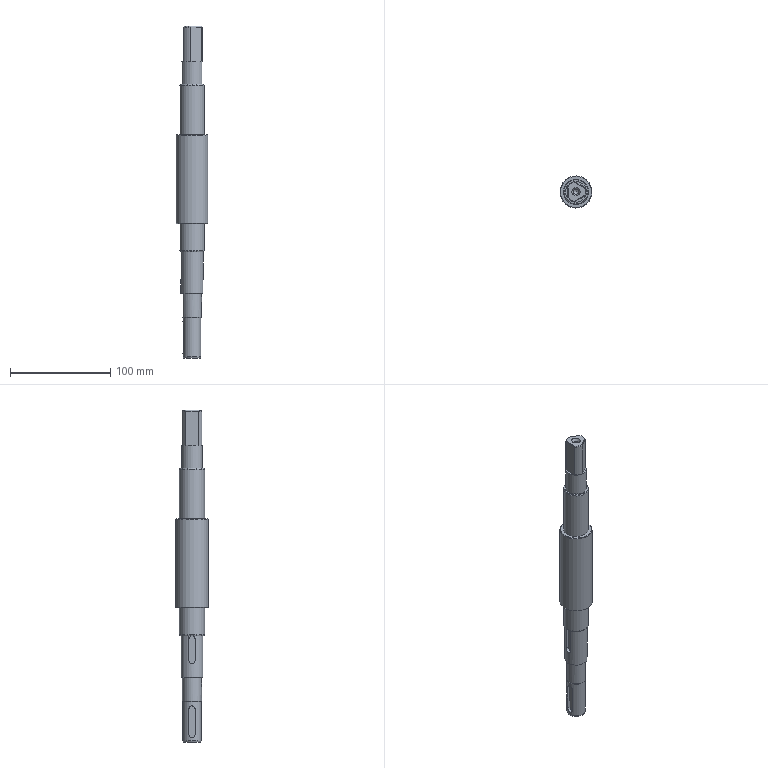Part | 1 solid | 57 faces | box 32 x 32 x 331.3 mm | volume 157834 mm3 | plane 24 | cylinder 19 | cone 14 | commonest cylinder face diameters 6 x4 5 x3 20 x3 22 x2 25 x2 4 x1
STEP:
#1=CARTESIAN_POINT('',(-1.,0.,-24.502));
#2=VERTEX_POINT('',#1);
#3=VERTEX_LOOP('',#2);
#4=FACE_BOUND('',#3,.T.);
#5=CARTESIAN_POINT('',(-1.,2.5,-23.));
#6=VERTEX_POINT('',#5);
#7=CARTESIAN_POINT('',(-1.,0.,-23.));
#8=DIRECTION('',(0.,0.,1.));
#9=DIRECTION('',(0.,1.,0.));
#10=AXIS2_PLACEMENT_3D('',#7,#8,#9);
#11=CIRCLE('',#10,2.5);
#12=EDGE_CURVE('',#6,#6,#11,.T.);
#13=ORIENTED_EDGE('',*,*,#12,.T.);
#14=EDGE_LOOP('',(#13));
#15=FACE_BOUND('',#14,.T.);
#16=CARTESIAN_POINT('',(-1.,0.,-23.));
#17=DIRECTION('',(0.,0.,1.));
#18=DIRECTION('',(0.,1.,0.));
#19=AXIS2_PLACEMENT_3D('',#16,#17,#18);
#20=CONICAL_SURFACE('',#19,2.5,1.03);
#21=ADVANCED_FACE('',(#4,#15),#20,.F.);
#22=ORIENTED_EDGE('',*,*,#12,.F.);
#23=EDGE_LOOP('',(#22));
#24=FACE_BOUND('',#23,.T.);
#25=CARTESIAN_POINT('',(-1.,2.5,-3.031));
#26=VERTEX_POINT('',#25);
#27=CARTESIAN_POINT('',(-1.,0.,-3.031));
#28=DIRECTION('',(0.,0.,1.));
#29=DIRECTION('',(0.,1.,0.));
#30=AXIS2_PLACEMENT_3D('',#27,#28,#29);
#31=CIRCLE('',#30,2.5);
#32=EDGE_CURVE('',#26,#26,#31,.F.);
#33=ORIENTED_EDGE('',*,*,#32,.F.);
#34=EDGE_LOOP('',(#33));
#35=FACE_BOUND('',#34,.T.);
#36=CARTESIAN_POINT('',(-1.,0.,0.));
#37=DIRECTION('',(0.,0.,1.));
#38=DIRECTION('',(0.,1.,0.));
#39=AXIS2_PLACEMENT_3D('',#36,#37,#38);
#40=CYLINDRICAL_SURFACE('',#39,2.5);
#41=ADVANCED_FACE('',(#24,#35),#40,.F.);
#42=ORIENTED_EDGE('',*,*,#32,.T.);
#43=EDGE_LOOP('',(#42));
#44=FACE_BOUND('',#43,.T.);
#45=CARTESIAN_POINT('',(-1.,4.25,0.));
#46=VERTEX_POINT('',#45);
#47=CARTESIAN_POINT('',(-1.,0.,0.));
#48=DIRECTION('',(0.,0.,1.));
#49=DIRECTION('',(0.,1.,0.));
#50=AXIS2_PLACEMENT_3D('',#47,#48,#49);
#51=CIRCLE('',#50,4.25);
#52=EDGE_CURVE('',#46,#46,#51,.T.);
#53=ORIENTED_EDGE('',*,*,#52,.T.);
#54=EDGE_LOOP('',(#53));
#55=FACE_BOUND('',#54,.T.);
#56=CARTESIAN_POINT('',(-1.,0.,0.));
#57=DIRECTION('',(0.,0.,1.));
#58=DIRECTION('',(0.,1.,0.));
#59=AXIS2_PLACEMENT_3D('',#56,#57,#58);
#60=CONICAL_SURFACE('',#59,4.25,0.5236);
#61=ADVANCED_FACE('',(#44,#55),#60,.F.);
#62=ORIENTED_EDGE('',*,*,#52,.F.);
#63=EDGE_LOOP('',(#62));
#64=FACE_BOUND('',#63,.T.);
#65=CARTESIAN_POINT('',(7.827,-3.603,0.));
#66=VERTEX_POINT('',#65);
#67=CARTESIAN_POINT('',(7.827,3.603,0.));
#68=VERTEX_POINT('',#67);
#69=CARTESIAN_POINT('',(-1.,0.,0.));
#70=DIRECTION('',(0.,0.,-1.));
#71=DIRECTION('',(0.,-1.,0.));
#72=AXIS2_PLACEMENT_3D('',#69,#70,#71);
#73=CIRCLE('',#72,9.534);
#74=EDGE_CURVE('',#66,#68,#73,.F.);
#75=ORIENTED_EDGE('',*,*,#74,.T.);
#76=CARTESIAN_POINT('',(-2.293,9.446,0.));
#77=VERTEX_POINT('',#76);
#78=CARTESIAN_POINT('',(2.767,6.524,0.));
#79=DIRECTION('',(-0.866,0.5,0.));
#80=VECTOR('',#79,1000.);
#81=LINE('',#78,#80);
#82=EDGE_CURVE('',#68,#77,#81,.T.);
#83=ORIENTED_EDGE('',*,*,#82,.T.);
#84=CARTESIAN_POINT('',(-8.534,5.842,0.));
#85=VERTEX_POINT('',#84);
#86=CARTESIAN_POINT('',(-1.,0.,0.));
#87=DIRECTION('',(0.,0.,-1.));
#88=DIRECTION('',(0.,-1.,0.));
#89=AXIS2_PLACEMENT_3D('',#86,#87,#88);
#90=CIRCLE('',#89,9.534);
#91=EDGE_CURVE('',#77,#85,#90,.F.);
#92=ORIENTED_EDGE('',*,*,#91,.T.);
#93=CARTESIAN_POINT('',(-8.534,-5.842,0.));
#94=VERTEX_POINT('',#93);
#95=CARTESIAN_POINT('',(-8.534,0.,0.));
#96=DIRECTION('',(0.,-1.,0.));
#97=VECTOR('',#96,1000.);
#98=LINE('',#95,#97);
#99=EDGE_CURVE('',#85,#94,#98,.T.);
#100=ORIENTED_EDGE('',*,*,#99,.T.);
#101=CARTESIAN_POINT('',(-2.293,-9.446,0.));
#102=VERTEX_POINT('',#101);
#103=CARTESIAN_POINT('',(-1.,0.,0.));
#104=DIRECTION('',(0.,0.,-1.));
#105=DIRECTION('',(0.,-1.,0.));
#106=AXIS2_PLACEMENT_3D('',#103,#104,#105);
#107=CIRCLE('',#106,9.534);
#108=EDGE_CURVE('',#94,#102,#107,.F.);
#109=ORIENTED_EDGE('',*,*,#108,.T.);
#110=CARTESIAN_POINT('',(2.767,-6.524,0.));
#111=DIRECTION('',(0.866,0.5,0.));
#112=VECTOR('',#111,1000.);
#113=LINE('',#110,#112);
#114=EDGE_CURVE('',#102,#66,#113,.T.);
#115=ORIENTED_EDGE('',*,*,#114,.T.);
#116=EDGE_LOOP('',(#75,#83,#92,#100,#109,#115));
#117=FACE_BOUND('',#116,.T.);
#118=CARTESIAN_POINT('',(-1.,0.,0.));
#119=DIRECTION('',(0.,0.,-1.));
#120=DIRECTION('',(0.,-1.,0.));
#121=AXIS2_PLACEMENT_3D('',#118,#119,#120);
#122=PLANE('',#121);
#123=ADVANCED_FACE('',(#64,#117),#122,.F.);
#124=CARTESIAN_POINT('',(-2.196,-9.928,-1.));
#125=VERTEX_POINT('',#124);
#126=CARTESIAN_POINT('',(-9.,-6.,-1.));
#127=VERTEX_POINT('',#126);
#128=CARTESIAN_POINT('',(-1.,0.,-1.));
#129=DIRECTION('',(0.,0.,-1.));
#130=DIRECTION('',(0.,-1.,0.));
#131=AXIS2_PLACEMENT_3D('',#128,#129,#130);
#132=CIRCLE('',#131,10.);
#133=EDGE_CURVE('',#125,#127,#132,.T.);
#134=ORIENTED_EDGE('',*,*,#133,.F.);
#135=CARTESIAN_POINT('',(-2.196,-9.928,-1.));
#136=CARTESIAN_POINT('',(-2.229,-9.768,-0.6666));
#137=CARTESIAN_POINT('',(-2.261,-9.607,-0.3332));
#138=CARTESIAN_POINT('',(-2.293,-9.446,0.));
#139=B_SPLINE_CURVE_WITH_KNOTS('',3,(#135,#136,#137,#138),.UNSPECIFIED.,.F.,.F.,(4,4),(0.,0.001115),.UNSPECIFIED.);
#140=EDGE_CURVE('',#125,#102,#139,.T.);
#141=ORIENTED_EDGE('',*,*,#140,.T.);
#142=ORIENTED_EDGE('',*,*,#108,.F.);
#143=CARTESIAN_POINT('',(-8.534,-5.842,0.));
#144=CARTESIAN_POINT('',(-8.689,-5.896,-0.3332));
#145=CARTESIAN_POINT('',(-8.845,-5.948,-0.6666));
#146=CARTESIAN_POINT('',(-9.,-6.,-1.));
#147=B_SPLINE_CURVE_WITH_KNOTS('',3,(#143,#144,#145,#146),.UNSPECIFIED.,.F.,.F.,(4,4),(0.,0.001115),.UNSPECIFIED.);
#148=EDGE_CURVE('',#94,#127,#147,.T.);
#149=ORIENTED_EDGE('',*,*,#148,.T.);
#150=EDGE_LOOP('',(#134,#141,#142,#149));
#151=FACE_BOUND('',#150,.T.);
#152=CARTESIAN_POINT('',(-1.,0.,0.));
#153=DIRECTION('',(0.,0.,-1.));
#154=DIRECTION('',(0.,-1.,0.));
#155=AXIS2_PLACEMENT_3D('',#152,#153,#154);
#156=CONICAL_SURFACE('',#155,9.534,0.4363);
#157=ADVANCED_FACE('',(#151),#156,.T.);
#158=CARTESIAN_POINT('',(8.196,-3.928,-1.));
#159=VERTEX_POINT('',#158);
#160=CARTESIAN_POINT('',(7.827,-3.603,0.));
#161=CARTESIAN_POINT('',(7.95,-3.711,-0.3332));
#162=CARTESIAN_POINT('',(8.074,-3.819,-0.6666));
#163=CARTESIAN_POINT('',(8.196,-3.928,-1.));
#164=B_SPLINE_CURVE_WITH_KNOTS('',3,(#160,#161,#162,#163),.UNSPECIFIED.,.F.,.F.,(4,4),(0.,0.001115),.UNSPECIFIED.);
#165=EDGE_CURVE('',#66,#159,#164,.T.);
#166=ORIENTED_EDGE('',*,*,#165,.F.);
#167=ORIENTED_EDGE('',*,*,#114,.F.);
#168=ORIENTED_EDGE('',*,*,#140,.F.);
#169=CARTESIAN_POINT('',(8.196,-3.928,-1.));
#170=DIRECTION('',(-0.866,-0.5,0.));
#171=VECTOR('',#170,1000.);
#172=LINE('',#169,#171);
#173=EDGE_CURVE('',#159,#125,#172,.T.);
#174=ORIENTED_EDGE('',*,*,#173,.F.);
#175=EDGE_LOOP('',(#166,#167,#168,#174));
#176=FACE_BOUND('',#175,.T.);
#177=CARTESIAN_POINT('',(8.196,-3.928,-1.));
#178=DIRECTION('',(-0.4532,0.7849,-0.4226));
#179=DIRECTION('',(-0.866,-0.5,0.));
#180=AXIS2_PLACEMENT_3D('',#177,#178,#179);
#181=PLANE('',#180);
#182=ADVANCED_FACE('',(#176),#181,.F.);
#183=CARTESIAN_POINT('',(8.196,3.928,-1.));
#184=VERTEX_POINT('',#183);
#185=CARTESIAN_POINT('',(-1.,0.,-1.));
#186=DIRECTION('',(0.,0.,-1.));
#187=DIRECTION('',(0.,-1.,0.));
#188=AXIS2_PLACEMENT_3D('',#185,#186,#187);
#189=CIRCLE('',#188,10.);
#190=EDGE_CURVE('',#184,#159,#189,.T.);
#191=ORIENTED_EDGE('',*,*,#190,.F.);
#192=CARTESIAN_POINT('',(8.196,3.928,-1.));
#193=CARTESIAN_POINT('',(8.074,3.819,-0.6666));
#194=CARTESIAN_POINT('',(7.95,3.711,-0.3332));
#195=CARTESIAN_POINT('',(7.827,3.603,0.));
#196=B_SPLINE_CURVE_WITH_KNOTS('',3,(#192,#193,#194,#195),.UNSPECIFIED.,.F.,.F.,(4,4),(0.,0.001115),.UNSPECIFIED.);
#197=EDGE_CURVE('',#184,#68,#196,.T.);
#198=ORIENTED_EDGE('',*,*,#197,.T.);
#199=ORIENTED_EDGE('',*,*,#74,.F.);
#200=ORIENTED_EDGE('',*,*,#165,.T.);
#201=EDGE_LOOP('',(#191,#198,#199,#200));
#202=FACE_BOUND('',#201,.T.);
#203=CARTESIAN_POINT('',(-1.,0.,0.));
#204=DIRECTION('',(0.,0.,-1.));
#205=DIRECTION('',(0.,-1.,0.));
#206=AXIS2_PLACEMENT_3D('',#203,#204,#205);
#207=CONICAL_SURFACE('',#206,9.534,0.4363);
#208=ADVANCED_FACE('',(#202),#207,.T.);
#209=CARTESIAN_POINT('',(-2.196,9.928,-1.));
#210=VERTEX_POINT('',#209);
#211=CARTESIAN_POINT('',(-2.293,9.446,0.));
#212=CARTESIAN_POINT('',(-2.261,9.607,-0.3332));
#213=CARTESIAN_POINT('',(-2.229,9.768,-0.6666));
#214=CARTESIAN_POINT('',(-2.196,9.928,-1.));
#215=B_SPLINE_CURVE_WITH_KNOTS('',3,(#211,#212,#213,#214),.UNSPECIFIED.,.F.,.F.,(4,4),(0.,0.001115),.UNSPECIFIED.);
#216=EDGE_CURVE('',#77,#210,#215,.T.);
#217=ORIENTED_EDGE('',*,*,#216,.F.);
#218=ORIENTED_EDGE('',*,*,#82,.F.);
#219=ORIENTED_EDGE('',*,*,#197,.F.);
#220=CARTESIAN_POINT('',(-2.196,9.928,-1.));
#221=DIRECTION('',(0.866,-0.5,0.));
#222=VECTOR('',#221,1000.);
#223=LINE('',#220,#222);
#224=EDGE_CURVE('',#210,#184,#223,.T.);
#225=ORIENTED_EDGE('',*,*,#224,.F.);
#226=EDGE_LOOP('',(#217,#218,#219,#225));
#227=FACE_BOUND('',#226,.T.);
#228=CARTESIAN_POINT('',(-2.196,9.928,-1.));
#229=DIRECTION('',(-0.4532,-0.7849,-0.4226));
#230=DIRECTION('',(0.866,-0.5,0.));
#231=AXIS2_PLACEMENT_3D('',#228,#229,#230);
#232=PLANE('',#231);
#233=ADVANCED_FACE('',(#227),#232,.F.);
#234=ORIENTED_EDGE('',*,*,#91,.F.);
#235=ORIENTED_EDGE('',*,*,#216,.T.);
#236=CARTESIAN_POINT('',(-9.,6.,-1.));
#237=VERTEX_POINT('',#236);
#238=CARTESIAN_POINT('',(-1.,0.,-1.));
#239=DIRECTION('',(0.,0.,-1.));
#240=DIRECTION('',(0.,-1.,0.));
#241=AXIS2_PLACEMENT_3D('',#238,#239,#240);
#242=CIRCLE('',#241,10.);
#243=EDGE_CURVE('',#237,#210,#242,.T.);
#244=ORIENTED_EDGE('',*,*,#243,.F.);
#245=CARTESIAN_POINT('',(-9.,6.,-1.));
#246=CARTESIAN_POINT('',(-8.845,5.948,-0.6666));
#247=CARTESIAN_POINT('',(-8.689,5.896,-0.3332));
#248=CARTESIAN_POINT('',(-8.534,5.842,0.));
#249=B_SPLINE_CURVE_WITH_KNOTS('',3,(#245,#246,#247,#248),.UNSPECIFIED.,.F.,.F.,(4,4),(0.,0.001115),.UNSPECIFIED.);
#250=EDGE_CURVE('',#237,#85,#249,.T.);
#251=ORIENTED_EDGE('',*,*,#250,.T.);
#252=EDGE_LOOP('',(#234,#235,#244,#251));
#253=FACE_BOUND('',#252,.T.);
#254=CARTESIAN_POINT('',(-1.,0.,0.));
#255=DIRECTION('',(0.,0.,-1.));
#256=DIRECTION('',(0.,-1.,0.));
#257=AXIS2_PLACEMENT_3D('',#254,#255,#256);
#258=CONICAL_SURFACE('',#257,9.534,0.4363);
#259=ADVANCED_FACE('',(#253),#258,.T.);
#260=ORIENTED_EDGE('',*,*,#148,.F.);
#261=ORIENTED_EDGE('',*,*,#99,.F.);
#262=ORIENTED_EDGE('',*,*,#250,.F.);
#263=CARTESIAN_POINT('',(-9.,-6.,-1.));
#264=DIRECTION('',(0.,1.,0.));
#265=VECTOR('',#264,1000.);
#266=LINE('',#263,#265);
#267=EDGE_CURVE('',#127,#237,#266,.T.);
#268=ORIENTED_EDGE('',*,*,#267,.F.);
#269=EDGE_LOOP('',(#260,#261,#262,#268));
#270=FACE_BOUND('',#269,.T.);
#271=CARTESIAN_POINT('',(-9.,-6.,-1.));
#272=DIRECTION('',(0.9063,0.,-0.4226));
#273=DIRECTION('',(0.,1.,0.));
#274=AXIS2_PLACEMENT_3D('',#271,#272,#273);
#275=PLANE('',#274);
#276=ADVANCED_FACE('',(#270),#275,.F.);
#277=CARTESIAN_POINT('',(-9.,-6.,-35.));
#278=VERTEX_POINT('',#277);
#279=CARTESIAN_POINT('',(-9.,-6.,-35.));
#280=DIRECTION('',(0.,0.,1.));
#281=VECTOR('',#280,1000.);
#282=LINE('',#279,#281);
#283=EDGE_CURVE('',#278,#127,#282,.T.);
#284=ORIENTED_EDGE('',*,*,#283,.F.);
#285=CARTESIAN_POINT('',(-2.196,-9.928,-35.));
#286=VERTEX_POINT('',#285);
#287=CARTESIAN_POINT('',(-1.,0.,-35.));
#288=DIRECTION('',(0.,0.,1.));
#289=DIRECTION('',(0.,1.,0.));
#290=AXIS2_PLACEMENT_3D('',#287,#288,#289);
#291=CIRCLE('',#290,10.);
#292=EDGE_CURVE('',#278,#286,#291,.T.);
#293=ORIENTED_EDGE('',*,*,#292,.T.);
#294=CARTESIAN_POINT('',(-2.196,-9.928,-35.));
#295=DIRECTION('',(0.,0.,1.));
#296=VECTOR('',#295,1000.);
#297=LINE('',#294,#296);
#298=EDGE_CURVE('',#286,#125,#297,.T.);
#299=ORIENTED_EDGE('',*,*,#298,.T.);
#300=ORIENTED_EDGE('',*,*,#133,.T.);
#301=EDGE_LOOP('',(#284,#293,#299,#300));
#302=FACE_BOUND('',#301,.T.);
#303=CARTESIAN_POINT('',(-1.,0.,0.));
#304=DIRECTION('',(0.,0.,1.));
#305=DIRECTION('',(0.,1.,0.));
#306=AXIS2_PLACEMENT_3D('',#303,#304,#305);
#307=CYLINDRICAL_SURFACE('',#306,10.);
#308=ADVANCED_FACE('',(#302),#307,.T.);
#309=CARTESIAN_POINT('',(8.196,-3.928,-35.));
#310=VERTEX_POINT('',#309);
#311=CARTESIAN_POINT('',(8.196,-3.928,-35.));
#312=DIRECTION('',(0.,0.,1.));
#313=VECTOR('',#312,1000.);
#314=LINE('',#311,#313);
#315=EDGE_CURVE('',#310,#159,#314,.T.);
#316=ORIENTED_EDGE('',*,*,#315,.T.);
#317=ORIENTED_EDGE('',*,*,#173,.T.);
#318=ORIENTED_EDGE('',*,*,#298,.F.);
#319=CARTESIAN_POINT('',(8.196,-3.928,-35.));
#320=DIRECTION('',(-0.866,-0.5,0.));
#321=VECTOR('',#320,1000.);
#322=LINE('',#319,#321);
#323=EDGE_CURVE('',#310,#286,#322,.T.);
#324=ORIENTED_EDGE('',*,*,#323,.F.);
#325=EDGE_LOOP('',(#316,#317,#318,#324));
#326=FACE_BOUND('',#325,.T.);
#327=CARTESIAN_POINT('',(8.196,-3.928,-35.));
#328=DIRECTION('',(-0.5,0.866,0.));
#329=DIRECTION('',(0.866,0.5,0.));
#330=AXIS2_PLACEMENT_3D('',#327,#328,#329);
#331=PLANE('',#330);
#332=ADVANCED_FACE('',(#326),#331,.F.);
#333=ORIENTED_EDGE('',*,*,#315,.F.);
#334=CARTESIAN_POINT('',(8.196,3.928,-35.));
#335=VERTEX_POINT('',#334);
#336=CARTESIAN_POINT('',(-1.,0.,-35.));
#337=DIRECTION('',(0.,0.,1.));
#338=DIRECTION('',(0.,1.,0.));
#339=AXIS2_PLACEMENT_3D('',#336,#337,#338);
#340=CIRCLE('',#339,10.);
#341=EDGE_CURVE('',#310,#335,#340,.T.);
#342=ORIENTED_EDGE('',*,*,#341,.T.);
#343=CARTESIAN_POINT('',(8.196,3.928,-35.));
#344=DIRECTION('',(0.,0.,1.));
#345=VECTOR('',#344,1000.);
#346=LINE('',#343,#345);
#347=EDGE_CURVE('',#335,#184,#346,.T.);
#348=ORIENTED_EDGE('',*,*,#347,.T.);
#349=ORIENTED_EDGE('',*,*,#190,.T.);
#350=EDGE_LOOP('',(#333,#342,#348,#349));
#351=FACE_BOUND('',#350,.T.);
#352=CARTESIAN_POINT('',(-1.,0.,0.));
#353=DIRECTION('',(0.,0.,1.));
#354=DIRECTION('',(0.,1.,0.));
#355=AXIS2_PLACEMENT_3D('',#352,#353,#354);
#356=CYLINDRICAL_SURFACE('',#355,10.);
#357=ADVANCED_FACE('',(#351),#356,.T.);
#358=CARTESIAN_POINT('',(-2.196,9.928,-35.));
#359=VERTEX_POINT('',#358);
#360=CARTESIAN_POINT('',(-2.196,9.928,-35.));
#361=DIRECTION('',(0.,0.,1.));
#362=VECTOR('',#361,1000.);
#363=LINE('',#360,#362);
#364=EDGE_CURVE('',#359,#210,#363,.T.);
#365=ORIENTED_EDGE('',*,*,#364,.T.);
#366=ORIENTED_EDGE('',*,*,#224,.T.);
#367=ORIENTED_EDGE('',*,*,#347,.F.);
#368=CARTESIAN_POINT('',(-2.196,9.928,-35.));
#369=DIRECTION('',(0.866,-0.5,0.));
#370=VECTOR('',#369,1000.);
#371=LINE('',#368,#370);
#372=EDGE_CURVE('',#359,#335,#371,.T.);
#373=ORIENTED_EDGE('',*,*,#372,.F.);
#374=EDGE_LOOP('',(#365,#366,#367,#373));
#375=FACE_BOUND('',#374,.T.);
#376=CARTESIAN_POINT('',(-2.196,9.928,-35.));
#377=DIRECTION('',(-0.5,-0.866,0.));
#378=DIRECTION('',(-0.866,0.5,0.));
#379=AXIS2_PLACEMENT_3D('',#376,#377,#378);
#380=PLANE('',#379);
#381=ADVANCED_FACE('',(#375),#380,.F.);
#382=ORIENTED_EDGE('',*,*,#364,.F.);
#383=CARTESIAN_POINT('',(-9.,6.,-35.));
#384=VERTEX_POINT('',#383);
#385=CARTESIAN_POINT('',(-1.,0.,-35.));
#386=DIRECTION('',(0.,0.,1.));
#387=DIRECTION('',(0.,1.,0.));
#388=AXIS2_PLACEMENT_3D('',#385,#386,#387);
#389=CIRCLE('',#388,10.);
#390=EDGE_CURVE('',#359,#384,#389,.T.);
#391=ORIENTED_EDGE('',*,*,#390,.T.);
#392=CARTESIAN_POINT('',(-9.,6.,-35.));
#393=DIRECTION('',(0.,0.,1.));
#394=VECTOR('',#393,1000.);
#395=LINE('',#392,#394);
#396=EDGE_CURVE('',#384,#237,#395,.T.);
#397=ORIENTED_EDGE('',*,*,#396,.T.);
#398=ORIENTED_EDGE('',*,*,#243,.T.);
#399=EDGE_LOOP('',(#382,#391,#397,#398));
#400=FACE_BOUND('',#399,.T.);
#401=CARTESIAN_POINT('',(-1.,0.,0.));
#402=DIRECTION('',(0.,0.,1.));
#403=DIRECTION('',(0.,1.,0.));
#404=AXIS2_PLACEMENT_3D('',#401,#402,#403);
#405=CYLINDRICAL_SURFACE('',#404,10.);
#406=ADVANCED_FACE('',(#400),#405,.T.);
#407=ORIENTED_EDGE('',*,*,#283,.T.);
#408=ORIENTED_EDGE('',*,*,#267,.T.);
#409=ORIENTED_EDGE('',*,*,#396,.F.);
#410=CARTESIAN_POINT('',(-9.,-6.,-35.));
#411=DIRECTION('',(0.,1.,0.));
#412=VECTOR('',#411,1000.);
#413=LINE('',#410,#412);
#414=EDGE_CURVE('',#278,#384,#413,.T.);
#415=ORIENTED_EDGE('',*,*,#414,.F.);
#416=EDGE_LOOP('',(#407,#408,#409,#415));
#417=FACE_BOUND('',#416,.T.);
#418=CARTESIAN_POINT('',(-9.,-6.,-35.));
#419=DIRECTION('',(1.,0.,0.));
#420=DIRECTION('',(0.,-1.,0.));
#421=AXIS2_PLACEMENT_3D('',#418,#419,#420);
#422=PLANE('',#421);
#423=ADVANCED_FACE('',(#417),#422,.F.);
#424=CARTESIAN_POINT('',(-1.,-10.4,-35.));
#425=VERTEX_POINT('',#424);
#426=CARTESIAN_POINT('',(-1.,0.,-35.));
#427=DIRECTION('',(0.,0.,1.));
#428=DIRECTION('',(0.,-1.,0.));
#429=AXIS2_PLACEMENT_3D('',#426,#427,#428);
#430=CIRCLE('',#429,10.4);
#431=EDGE_CURVE('',#425,#425,#430,.F.);
#432=ORIENTED_EDGE('',*,*,#431,.F.);
#433=EDGE_LOOP('',(#432));
#434=FACE_BOUND('',#433,.T.);
#435=ORIENTED_EDGE('',*,*,#414,.T.);
#436=ORIENTED_EDGE('',*,*,#390,.F.);
#437=ORIENTED_EDGE('',*,*,#372,.T.);
#438=ORIENTED_EDGE('',*,*,#341,.F.);
#439=ORIENTED_EDGE('',*,*,#323,.T.);
#440=ORIENTED_EDGE('',*,*,#292,.F.);
#441=EDGE_LOOP('',(#435,#436,#437,#438,#439,#440));
#442=FACE_BOUND('',#441,.T.);
#443=CARTESIAN_POINT('',(-1.,0.,-35.));
#444=DIRECTION('',(0.,0.,1.));
#445=DIRECTION('',(0.,1.,0.));
#446=AXIS2_PLACEMENT_3D('',#443,#444,#445);
#447=PLANE('',#446);
#448=ADVANCED_FACE('',(#434,#442),#447,.T.);
#449=CARTESIAN_POINT('',(-1.,-10.4,-58.));
#450=VERTEX_POINT('',#449);
#451=CARTESIAN_POINT('',(-1.,0.,-58.));
#452=DIRECTION('',(0.,0.,-1.));
#453=DIRECTION('',(0.,-1.,0.));
#454=AXIS2_PLACEMENT_3D('',#451,#452,#453);
#455=CIRCLE('',#454,10.4);
#456=EDGE_CURVE('',#450,#450,#455,.F.);
#457=ORIENTED_EDGE('',*,*,#456,.T.);
#458=EDGE_LOOP('',(#457));
#459=FACE_BOUND('',#458,.T.);
#460=ORIENTED_EDGE('',*,*,#431,.T.);
#461=EDGE_LOOP('',(#460));
#462=FACE_BOUND('',#461,.T.);
#463=CARTESIAN_POINT('',(-1.,0.,-5.584));
#464=DIRECTION('',(0.,0.,-1.));
#465=DIRECTION('',(0.,-1.,0.));
#466=AXIS2_PLACEMENT_3D('',#463,#464,#465);
#467=CYLINDRICAL_SURFACE('',#466,10.4);
#468=ADVANCED_FACE('',(#459,#462),#467,.T.);
#469=CARTESIAN_POINT('',(-1.,-12.034,-58.));
#470=VERTEX_POINT('',#469);
#471=CARTESIAN_POINT('',(-1.,0.,-58.));
#472=DIRECTION('',(0.,0.,-1.));
#473=DIRECTION('',(0.,-1.,0.));
#474=AXIS2_PLACEMENT_3D('',#471,#472,#473);
#475=CIRCLE('',#474,12.034);
#476=EDGE_CURVE('',#470,#470,#475,.F.);
#477=ORIENTED_EDGE('',*,*,#476,.T.);
#478=EDGE_LOOP('',(#477));
#479=FACE_BOUND('',#478,.T.);
#480=ORIENTED_EDGE('',*,*,#456,.F.);
#481=EDGE_LOOP('',(#480));
#482=FACE_BOUND('',#481,.T.);
#483=CARTESIAN_POINT('',(-11.,0.,-58.));
#484=DIRECTION('',(0.,0.,-1.));
#485=DIRECTION('',(0.,-1.,0.));
#486=AXIS2_PLACEMENT_3D('',#483,#484,#485);
#487=PLANE('',#486);
#488=ADVANCED_FACE('',(#479,#482),#487,.F.);
#489=CARTESIAN_POINT('',(-1.,9.,-291.3));
#490=VERTEX_POINT('',#489);
#491=CARTESIAN_POINT('',(-1.,0.,-291.3));
#492=DIRECTION('',(0.,0.,1.));
#493=DIRECTION('',(0.,1.,0.));
#494=AXIS2_PLACEMENT_3D('',#491,#492,#493);
#495=CIRCLE('',#494,9.);
#496=EDGE_CURVE('',#490,#490,#495,.T.);
#497=ORIENTED_EDGE('',*,*,#496,.F.);
#498=EDGE_LOOP('',(#497));
#499=FACE_BOUND('',#498,.T.);
#500=CARTESIAN_POINT('',(-1.,9.,-330.3));
#501=VERTEX_POINT('',#500);
#502=CARTESIAN_POINT('',(-1.,0.,-330.3));
#503=DIRECTION('',(0.,0.,1.));
#504=DIRECTION('',(0.,1.,0.));
#505=AXIS2_PLACEMENT_3D('',#502,#503,#504);
#506=CIRCLE('',#505,9.);
#507=EDGE_CURVE('',#501,#501,#506,.T.);
#508=ORIENTED_EDGE('',*,*,#507,.T.);
#509=EDGE_LOOP('',(#508));
#510=FACE_BOUND('',#509,.T.);
#511=CARTESIAN_POINT('',(-9.485,3.,-298.3));
#512=VERTEX_POINT('',#511);
#513=CARTESIAN_POINT('',(-9.485,3.,-324.3));
#514=VERTEX_POINT('',#513);
#515=CARTESIAN_POINT('',(-9.485,3.,0.));
#516=DIRECTION('',(0.,0.,1.));
#517=VECTOR('',#516,1000.);
#518=LINE('',#515,#517);
#519=EDGE_CURVE('',#512,#514,#518,.F.);
#520=ORIENTED_EDGE('',*,*,#519,.F.);
#521=CARTESIAN_POINT('',(-9.485,-3.,-298.3));
#522=VERTEX_POINT('',#521);
#523=CARTESIAN_POINT('',(-9.485,-3.,-298.3));
#524=CARTESIAN_POINT('',(-9.485,-3.,-297.501));
#525=CARTESIAN_POINT('',(-9.75,-2.35,-295.957));
#526=CARTESIAN_POINT('',(-10.125,-0.005191,-294.972));
#527=CARTESIAN_POINT('',(-9.75,2.351,-295.956));
#528=CARTESIAN_POINT('',(-9.485,3.,-297.501));
#529=CARTESIAN_POINT('',(-9.485,3.,-298.3));
#530=B_SPLINE_CURVE_WITH_KNOTS('',3,(#523,#524,#525,#526,#527,#528,#529),.UNSPECIFIED.,.F.,.F.,(4,1,1,1,4),(0.,0.002361,0.004722,0.007083,0.009444),.UNSPECIFIED.);
#531=EDGE_CURVE('',#522,#512,#530,.T.);
#532=ORIENTED_EDGE('',*,*,#531,.F.);
#533=CARTESIAN_POINT('',(-9.485,-3.,-324.3));
#534=VERTEX_POINT('',#533);
#535=CARTESIAN_POINT('',(-9.485,-3.,0.));
#536=DIRECTION('',(0.,0.,1.));
#537=VECTOR('',#536,1000.);
#538=LINE('',#535,#537);
#539=EDGE_CURVE('',#522,#534,#538,.F.);
#540=ORIENTED_EDGE('',*,*,#539,.T.);
#541=CARTESIAN_POINT('',(-9.485,3.,-324.3));
#542=CARTESIAN_POINT('',(-9.485,3.,-325.099));
#543=CARTESIAN_POINT('',(-9.75,2.35,-326.643));
#544=CARTESIAN_POINT('',(-10.125,0.005191,-327.628));
#545=CARTESIAN_POINT('',(-9.75,-2.351,-326.644));
#546=CARTESIAN_POINT('',(-9.485,-3.,-325.099));
#547=CARTESIAN_POINT('',(-9.485,-3.,-324.3));
#548=B_SPLINE_CURVE_WITH_KNOTS('',3,(#541,#542,#543,#544,#545,#546,#547),.UNSPECIFIED.,.F.,.F.,(4,1,1,1,4),(0.,0.002361,0.004722,0.007083,0.009444),.UNSPECIFIED.);
#549=EDGE_CURVE('',#514,#534,#548,.T.);
#550=ORIENTED_EDGE('',*,*,#549,.F.);
#551=EDGE_LOOP('',(#520,#532,#540,#550));
#552=FACE_BOUND('',#551,.T.);
#553=CARTESIAN_POINT('',(-1.,0.,0.));
#554=DIRECTION('',(0.,0.,1.));
#555=DIRECTION('',(0.,1.,0.));
#556=AXIS2_PLACEMENT_3D('',#553,#554,#555);
#557=CYLINDRICAL_SURFACE('',#556,9.);
#558=ADVANCED_FACE('',(#499,#510,#552),#557,.T.);
#559=CARTESIAN_POINT('',(9.712,2.5,-255.3));
#560=VERTEX_POINT('',#559);
#561=CARTESIAN_POINT('',(9.712,2.5,-266.723));
#562=VERTEX_POINT('',#561);
#563=CARTESIAN_POINT('',(9.712,2.5,0.));
#564=DIRECTION('',(0.,0.,1.));
#565=VECTOR('',#564,1000.);
#566=LINE('',#563,#565);
#567=EDGE_CURVE('',#560,#562,#566,.F.);
#568=ORIENTED_EDGE('',*,*,#567,.T.);
#569=CARTESIAN_POINT('',(9.712,-2.5,-266.723));
#570=VERTEX_POINT('',#569);
#571=CARTESIAN_POINT('',(-1.,0.,-266.723));
#572=DIRECTION('',(0.,0.,1.));
#573=DIRECTION('',(0.,1.,0.));
#574=AXIS2_PLACEMENT_3D('',#571,#572,#573);
#575=CIRCLE('',#574,11.);
#576=EDGE_CURVE('',#562,#570,#575,.T.);
#577=ORIENTED_EDGE('',*,*,#576,.T.);
#578=CARTESIAN_POINT('',(9.712,-2.5,-255.3));
#579=VERTEX_POINT('',#578);
#580=CARTESIAN_POINT('',(9.712,-2.5,0.));
#581=DIRECTION('',(0.,0.,1.));
#582=VECTOR('',#581,1000.);
#583=LINE('',#580,#582);
#584=EDGE_CURVE('',#570,#579,#583,.T.);
#585=ORIENTED_EDGE('',*,*,#584,.T.);
#586=CARTESIAN_POINT('',(9.712,-2.5,-255.3));
#587=CARTESIAN_POINT('',(9.712,-2.5,-254.637));
#588=CARTESIAN_POINT('',(9.858,-1.958,-253.346));
#589=CARTESIAN_POINT('',(10.071,-0.00331,-252.527));
#590=CARTESIAN_POINT('',(9.858,1.959,-253.344));
#591=CARTESIAN_POINT('',(9.712,2.5,-254.637));
#592=CARTESIAN_POINT('',(9.712,2.5,-255.3));
#593=B_SPLINE_CURVE_WITH_KNOTS('',3,(#586,#587,#588,#589,#590,#591,#592),.UNSPECIFIED.,.F.,.F.,(4,1,1,1,4),(0.,0.00196,0.00392,0.00588,0.00784),.UNSPECIFIED.);
#594=EDGE_CURVE('',#579,#560,#593,.T.);
#595=ORIENTED_EDGE('',*,*,#594,.T.);
#596=EDGE_LOOP('',(#568,#577,#585,#595));
#597=FACE_BOUND('',#596,.T.);
#598=CARTESIAN_POINT('',(-11.583,3.,-228.3));
#599=VERTEX_POINT('',#598);
#600=CARTESIAN_POINT('',(-11.583,3.,-250.3));
#601=VERTEX_POINT('',#600);
#602=CARTESIAN_POINT('',(-11.583,3.,0.));
#603=DIRECTION('',(0.,0.,1.));
#604=VECTOR('',#603,1000.);
#605=LINE('',#602,#604);
#606=EDGE_CURVE('',#599,#601,#605,.F.);
#607=ORIENTED_EDGE('',*,*,#606,.F.);
#608=CARTESIAN_POINT('',(-12.,0.,-225.3));
#609=VERTEX_POINT('',#608);
#610=CARTESIAN_POINT('',(-12.,0.,-225.3));
#611=CARTESIAN_POINT('',(-12.,0.7863,-225.3));
#612=CARTESIAN_POINT('',(-11.795,2.35,-225.956));
#613=CARTESIAN_POINT('',(-11.583,3.,-227.504));
#614=CARTESIAN_POINT('',(-11.583,3.,-228.3));
#615=B_SPLINE_CURVE_WITH_KNOTS('',3,(#610,#611,#612,#613,#614),.UNSPECIFIED.,.F.,.F.,(4,1,4),(0.004713,0.007067,0.009421),.UNSPECIFIED.);
#616=EDGE_CURVE('',#609,#599,#615,.T.);
#617=ORIENTED_EDGE('',*,*,#616,.F.);
#618=CARTESIAN_POINT('',(-1.,0.,-225.3));
#619=DIRECTION('',(0.,0.,1.));
#620=DIRECTION('',(0.,1.,0.));
#621=AXIS2_PLACEMENT_3D('',#618,#619,#620);
#622=CIRCLE('',#621,11.);
#623=EDGE_CURVE('',#609,#609,#622,.T.);
#624=ORIENTED_EDGE('',*,*,#623,.F.);
#625=CARTESIAN_POINT('',(-11.583,-3.,-228.3));
#626=VERTEX_POINT('',#625);
#627=CARTESIAN_POINT('',(-11.583,-3.,-228.3));
#628=CARTESIAN_POINT('',(-11.583,-3.,-227.503));
#629=CARTESIAN_POINT('',(-11.796,-2.347,-225.954));
#630=CARTESIAN_POINT('',(-12.,-0.7872,-225.3));
#631=CARTESIAN_POINT('',(-12.,0.,-225.3));
#632=B_SPLINE_CURVE_WITH_KNOTS('',3,(#627,#628,#629,#630,#631),.UNSPECIFIED.,.F.,.F.,(4,1,4),(0.,0.002357,0.004713),.UNSPECIFIED.);
#633=EDGE_CURVE('',#626,#609,#632,.T.);
#634=ORIENTED_EDGE('',*,*,#633,.F.);
#635=CARTESIAN_POINT('',(-11.583,-3.,-250.3));
#636=VERTEX_POINT('',#635);
#637=CARTESIAN_POINT('',(-11.583,-3.,0.));
#638=DIRECTION('',(0.,0.,1.));
#639=VECTOR('',#638,1000.);
#640=LINE('',#637,#639);
#641=EDGE_CURVE('',#626,#636,#640,.F.);
#642=ORIENTED_EDGE('',*,*,#641,.T.);
#643=CARTESIAN_POINT('',(-11.583,3.,-250.3));
#644=CARTESIAN_POINT('',(-11.583,3.,-251.097));
#645=CARTESIAN_POINT('',(-11.796,2.35,-252.644));
#646=CARTESIAN_POINT('',(-12.102,0.004455,-253.627));
#647=CARTESIAN_POINT('',(-11.796,-2.351,-252.646));
#648=CARTESIAN_POINT('',(-11.583,-3.,-251.097));
#649=CARTESIAN_POINT('',(-11.583,-3.,-250.3));
#650=B_SPLINE_CURVE_WITH_KNOTS('',3,(#643,#644,#645,#646,#647,#648,#649),.UNSPECIFIED.,.F.,.F.,(4,1,1,1,4),(0.,0.002355,0.004711,0.007066,0.009421),.UNSPECIFIED.);
#651=EDGE_CURVE('',#601,#636,#650,.T.);
#652=ORIENTED_EDGE('',*,*,#651,.F.);
#653=EDGE_LOOP('',(#607,#617,#624,#634,#642,#652));
#654=FACE_BOUND('',#653,.T.);
#655=CARTESIAN_POINT('',(-1.,0.,0.));
#656=DIRECTION('',(0.,0.,1.));
#657=DIRECTION('',(0.,1.,0.));
#658=AXIS2_PLACEMENT_3D('',#655,#656,#657);
#659=CYLINDRICAL_SURFACE('',#658,11.);
#660=ADVANCED_FACE('',(#597,#654),#659,.T.);
#661=CARTESIAN_POINT('',(-1.,-12.5,-59.));
#662=VERTEX_POINT('',#661);
#663=CARTESIAN_POINT('',(-1.,0.,-59.));
#664=DIRECTION('',(0.,0.,-1.));
#665=DIRECTION('',(0.,-1.,0.));
#666=AXIS2_PLACEMENT_3D('',#663,#664,#665);
#667=CIRCLE('',#666,12.5);
#668=EDGE_CURVE('',#662,#662,#667,.T.);
#669=ORIENTED_EDGE('',*,*,#668,.T.);
#670=EDGE_LOOP('',(#669));
#671=FACE_BOUND('',#670,.T.);
#672=CARTESIAN_POINT('',(-1.,12.5,-108.3));
#673=VERTEX_POINT('',#672);
#674=CARTESIAN_POINT('',(-1.,0.,-108.3));
#675=DIRECTION('',(0.,0.,1.));
#676=DIRECTION('',(0.,1.,0.));
#677=AXIS2_PLACEMENT_3D('',#674,#675,#676);
#678=CIRCLE('',#677,12.5);
#679=EDGE_CURVE('',#673,#673,#678,.T.);
#680=ORIENTED_EDGE('',*,*,#679,.T.);
#681=EDGE_LOOP('',(#680));
#682=FACE_BOUND('',#681,.T.);
#683=CARTESIAN_POINT('',(-1.,0.,0.));
#684=DIRECTION('',(0.,0.,1.));
#685=DIRECTION('',(0.,1.,0.));
#686=AXIS2_PLACEMENT_3D('',#683,#684,#685);
#687=CYLINDRICAL_SURFACE('',#686,12.5);
#688=ADVANCED_FACE('',(#671,#682),#687,.T.);
#689=CARTESIAN_POINT('',(-1.,-15.5,-108.3));
#690=VERTEX_POINT('',#689);
#691=CARTESIAN_POINT('',(-1.,0.,-108.3));
#692=DIRECTION('',(0.,0.,-1.));
#693=DIRECTION('',(0.,-1.,0.));
#694=AXIS2_PLACEMENT_3D('',#691,#692,#693);
#695=CIRCLE('',#694,15.5);
#696=EDGE_CURVE('',#690,#690,#695,.F.);
#697=ORIENTED_EDGE('',*,*,#696,.T.);
#698=EDGE_LOOP('',(#697));
#699=FACE_BOUND('',#698,.T.);
#700=ORIENTED_EDGE('',*,*,#679,.F.);
#701=EDGE_LOOP('',(#700));
#702=FACE_BOUND('',#701,.T.);
#703=CARTESIAN_POINT('',(-13.5,0.,-108.3));
#704=DIRECTION('',(0.,0.,-1.));
#705=DIRECTION('',(0.,-1.,0.));
#706=AXIS2_PLACEMENT_3D('',#703,#704,#705);
#707=PLANE('',#706);
#708=ADVANCED_FACE('',(#699,#702),#707,.F.);
#709=CARTESIAN_POINT('',(-1.,-16.,-108.8));
#710=VERTEX_POINT('',#709);
#711=CARTESIAN_POINT('',(-1.,0.,-108.8));
#712=DIRECTION('',(0.,0.,-1.));
#713=DIRECTION('',(0.,-1.,0.));
#714=AXIS2_PLACEMENT_3D('',#711,#712,#713);
#715=CIRCLE('',#714,16.);
#716=EDGE_CURVE('',#710,#710,#715,.T.);
#717=ORIENTED_EDGE('',*,*,#716,.T.);
#718=EDGE_LOOP('',(#717));
#719=FACE_BOUND('',#718,.T.);
#720=CARTESIAN_POINT('',(-1.,16.,-196.8));
#721=VERTEX_POINT('',#720);
#722=CARTESIAN_POINT('',(-1.,0.,-196.8));
#723=DIRECTION('',(0.,0.,1.));
#724=DIRECTION('',(0.,1.,0.));
#725=AXIS2_PLACEMENT_3D('',#722,#723,#724);
#726=CIRCLE('',#725,16.);
#727=EDGE_CURVE('',#721,#721,#726,.T.);
#728=ORIENTED_EDGE('',*,*,#727,.T.);
#729=EDGE_LOOP('',(#728));
#730=FACE_BOUND('',#729,.T.);
#731=CARTESIAN_POINT('',(-1.,0.,0.));
#732=DIRECTION('',(0.,0.,1.));
#733=DIRECTION('',(0.,1.,0.));
#734=AXIS2_PLACEMENT_3D('',#731,#732,#733);
#735=CYLINDRICAL_SURFACE('',#734,16.);
#736=ADVANCED_FACE('',(#719,#730),#735,.T.);
#737=CARTESIAN_POINT('',(-1.,15.5,-197.3));
#738=VERTEX_POINT('',#737);
#739=CARTESIAN_POINT('',(-1.,0.,-197.3));
#740=DIRECTION('',(0.,0.,1.));
#741=DIRECTION('',(0.,1.,0.));
#742=AXIS2_PLACEMENT_3D('',#739,#740,#741);
#743=CIRCLE('',#742,15.5);
#744=EDGE_CURVE('',#738,#738,#743,.F.);
#745=ORIENTED_EDGE('',*,*,#744,.T.);
#746=EDGE_LOOP('',(#745));
#747=FACE_BOUND('',#746,.T.);
#748=CARTESIAN_POINT('',(-1.,12.5,-197.3));
#749=VERTEX_POINT('',#748);
#750=CARTESIAN_POINT('',(-1.,0.,-197.3));
#751=DIRECTION('',(0.,0.,1.));
#752=DIRECTION('',(0.,1.,0.));
#753=AXIS2_PLACEMENT_3D('',#750,#751,#752);
#754=CIRCLE('',#753,12.5);
#755=EDGE_CURVE('',#749,#749,#754,.T.);
#756=ORIENTED_EDGE('',*,*,#755,.T.);
#757=EDGE_LOOP('',(#756));
#758=FACE_BOUND('',#757,.T.);
#759=CARTESIAN_POINT('',(-17.,0.,-197.3));
#760=DIRECTION('',(0.,0.,1.));
#761=DIRECTION('',(0.,1.,0.));
#762=AXIS2_PLACEMENT_3D('',#759,#760,#761);
#763=PLANE('',#762);
#764=ADVANCED_FACE('',(#747,#758),#763,.F.);
#765=CARTESIAN_POINT('',(-1.,12.5,-224.3));
#766=VERTEX_POINT('',#765);
#767=CARTESIAN_POINT('',(-1.,0.,-224.3));
#768=DIRECTION('',(0.,0.,1.));
#769=DIRECTION('',(0.,1.,0.));
#770=AXIS2_PLACEMENT_3D('',#767,#768,#769);
#771=CIRCLE('',#770,12.5);
#772=EDGE_CURVE('',#766,#766,#771,.T.);
#773=ORIENTED_EDGE('',*,*,#772,.T.);
#774=EDGE_LOOP('',(#773));
#775=FACE_BOUND('',#774,.T.);
#776=ORIENTED_EDGE('',*,*,#755,.F.);
#777=EDGE_LOOP('',(#776));
#778=FACE_BOUND('',#777,.T.);
#779=CARTESIAN_POINT('',(-1.,0.,0.));
#780=DIRECTION('',(0.,0.,1.));
#781=DIRECTION('',(0.,1.,0.));
#782=AXIS2_PLACEMENT_3D('',#779,#780,#781);
#783=CYLINDRICAL_SURFACE('',#782,12.5);
#784=ADVANCED_FACE('',(#775,#778),#783,.T.);
#785=CARTESIAN_POINT('',(-1.,12.034,-225.3));
#786=VERTEX_POINT('',#785);
#787=CARTESIAN_POINT('',(-1.,0.,-225.3));
#788=DIRECTION('',(0.,0.,1.));
#789=DIRECTION('',(0.,1.,0.));
#790=AXIS2_PLACEMENT_3D('',#787,#788,#789);
#791=CIRCLE('',#790,12.034);
#792=EDGE_CURVE('',#786,#786,#791,.F.);
#793=ORIENTED_EDGE('',*,*,#792,.T.);
#794=EDGE_LOOP('',(#793));
#795=FACE_BOUND('',#794,.T.);
#796=ORIENTED_EDGE('',*,*,#623,.T.);
#797=EDGE_LOOP('',(#796));
#798=FACE_BOUND('',#797,.T.);
#799=CARTESIAN_POINT('',(-13.5,0.,-225.3));
#800=DIRECTION('',(0.,0.,1.));
#801=DIRECTION('',(0.,1.,0.));
#802=AXIS2_PLACEMENT_3D('',#799,#800,#801);
#803=PLANE('',#802);
#804=ADVANCED_FACE('',(#795,#798),#803,.F.);
#805=CARTESIAN_POINT('',(8.682,-2.5,-267.3));
#806=VERTEX_POINT('',#805);
#807=CARTESIAN_POINT('',(8.165,-2.5,-267.3));
#808=VERTEX_POINT('',#807);
#809=CARTESIAN_POINT('',(17.5,-2.5,-267.3));
#810=DIRECTION('',(-1.,0.,0.));
#811=VECTOR('',#810,1000.);
#812=LINE('',#809,#811);
#813=EDGE_CURVE('',#806,#808,#812,.T.);
#814=ORIENTED_EDGE('',*,*,#813,.F.);
#815=CARTESIAN_POINT('',(8.682,2.5,-267.3));
#816=VERTEX_POINT('',#815);
#817=CARTESIAN_POINT('',(-1.,0.,-267.3));
#818=DIRECTION('',(0.,0.,1.));
#819=DIRECTION('',(0.,1.,0.));
#820=AXIS2_PLACEMENT_3D('',#817,#818,#819);
#821=CIRCLE('',#820,10.);
#822=EDGE_CURVE('',#806,#816,#821,.F.);
#823=ORIENTED_EDGE('',*,*,#822,.T.);
#824=CARTESIAN_POINT('',(8.165,2.5,-267.3));
#825=VERTEX_POINT('',#824);
#826=CARTESIAN_POINT('',(17.5,2.5,-267.3));
#827=DIRECTION('',(-1.,0.,0.));
#828=VECTOR('',#827,1000.);
#829=LINE('',#826,#828);
#830=EDGE_CURVE('',#816,#825,#829,.T.);
#831=ORIENTED_EDGE('',*,*,#830,.T.);
#832=CARTESIAN_POINT('',(-1.,0.,-267.3));
#833=DIRECTION('',(0.,0.,1.));
#834=DIRECTION('',(0.,1.,0.));
#835=AXIS2_PLACEMENT_3D('',#832,#833,#834);
#836=CIRCLE('',#835,9.5);
#837=EDGE_CURVE('',#825,#808,#836,.T.);
#838=ORIENTED_EDGE('',*,*,#837,.T.);
#839=EDGE_LOOP('',(#814,#823,#831,#838));
#840=FACE_BOUND('',#839,.T.);
#841=CARTESIAN_POINT('',(-12.,0.,-267.3));
#842=DIRECTION('',(0.,0.,1.));
#843=DIRECTION('',(0.,1.,0.));
#844=AXIS2_PLACEMENT_3D('',#841,#842,#843);
#845=PLANE('',#844);
#846=ADVANCED_FACE('',(#840),#845,.F.);
#847=CARTESIAN_POINT('',(-1.,9.5,-290.8));
#848=VERTEX_POINT('',#847);
#849=CARTESIAN_POINT('',(-1.,0.,-290.8));
#850=DIRECTION('',(0.,0.,1.));
#851=DIRECTION('',(0.,1.,0.));
#852=AXIS2_PLACEMENT_3D('',#849,#850,#851);
#853=CIRCLE('',#852,9.5);
#854=EDGE_CURVE('',#848,#848,#853,.T.);
#855=ORIENTED_EDGE('',*,*,#854,.T.);
#856=EDGE_LOOP('',(#855));
#857=FACE_BOUND('',#856,.T.);
#858=ORIENTED_EDGE('',*,*,#837,.F.);
#859=CARTESIAN_POINT('',(8.165,2.5,-267.3));
#860=CARTESIAN_POINT('',(8.165,2.5,-267.964));
#861=CARTESIAN_POINT('',(8.336,1.958,-269.254));
#862=CARTESIAN_POINT('',(8.582,0.003623,-270.073));
#863=CARTESIAN_POINT('',(8.336,-1.959,-269.255));
#864=CARTESIAN_POINT('',(8.165,-2.5,-267.964));
#865=CARTESIAN_POINT('',(8.165,-2.5,-267.3));
#866=B_SPLINE_CURVE_WITH_KNOTS('',3,(#859,#860,#861,#862,#863,#864,#865),.UNSPECIFIED.,.F.,.F.,(4,1,1,1,4),(0.,0.001962,0.003924,0.005886,0.007848),.UNSPECIFIED.);
#867=EDGE_CURVE('',#825,#808,#866,.T.);
#868=ORIENTED_EDGE('',*,*,#867,.T.);
#869=EDGE_LOOP('',(#858,#868));
#870=FACE_BOUND('',#869,.T.);
#871=CARTESIAN_POINT('',(-1.,0.,0.));
#872=DIRECTION('',(0.,0.,1.));
#873=DIRECTION('',(0.,1.,0.));
#874=AXIS2_PLACEMENT_3D('',#871,#872,#873);
#875=CYLINDRICAL_SURFACE('',#874,9.5);
#876=ADVANCED_FACE('',(#857,#870),#875,.T.);
#877=CARTESIAN_POINT('',(-1.,9.267,-291.3));
#878=VERTEX_POINT('',#877);
#879=CARTESIAN_POINT('',(-1.,0.,-291.3));
#880=DIRECTION('',(0.,0.,1.));
#881=DIRECTION('',(0.,1.,0.));
#882=AXIS2_PLACEMENT_3D('',#879,#880,#881);
#883=CIRCLE('',#882,9.267);
#884=EDGE_CURVE('',#878,#878,#883,.F.);
#885=ORIENTED_EDGE('',*,*,#884,.T.);
#886=EDGE_LOOP('',(#885));
#887=FACE_BOUND('',#886,.T.);
#888=ORIENTED_EDGE('',*,*,#496,.T.);
#889=EDGE_LOOP('',(#888));
#890=FACE_BOUND('',#889,.T.);
#891=CARTESIAN_POINT('',(-10.5,0.,-291.3));
#892=DIRECTION('',(0.,0.,1.));
#893=DIRECTION('',(0.,1.,0.));
#894=AXIS2_PLACEMENT_3D('',#891,#892,#893);
#895=PLANE('',#894);
#896=ADVANCED_FACE('',(#887,#890),#895,.F.);
#897=CARTESIAN_POINT('',(-1.,-4.25,-331.3));
#898=VERTEX_POINT('',#897);
#899=CARTESIAN_POINT('',(-1.,0.,-331.3));
#900=DIRECTION('',(0.,0.,-1.));
#901=DIRECTION('',(0.,-1.,0.));
#902=AXIS2_PLACEMENT_3D('',#899,#900,#901);
#903=CIRCLE('',#902,4.25);
#904=EDGE_CURVE('',#898,#898,#903,.T.);
#905=ORIENTED_EDGE('',*,*,#904,.F.);
#906=EDGE_LOOP('',(#905));
#907=FACE_BOUND('',#906,.T.);
#908=CARTESIAN_POINT('',(-1.,8.534,-331.3));
#909=VERTEX_POINT('',#908);
#910=CARTESIAN_POINT('',(-1.,0.,-331.3));
#911=DIRECTION('',(0.,0.,1.));
#912=DIRECTION('',(0.,1.,0.));
#913=AXIS2_PLACEMENT_3D('',#910,#911,#912);
#914=CIRCLE('',#913,8.534);
#915=EDGE_CURVE('',#909,#909,#914,.F.);
#916=ORIENTED_EDGE('',*,*,#915,.T.);
#917=EDGE_LOOP('',(#916));
#918=FACE_BOUND('',#917,.T.);
#919=CARTESIAN_POINT('',(-10.,0.,-331.3));
#920=DIRECTION('',(0.,0.,1.));
#921=DIRECTION('',(0.,1.,0.));
#922=AXIS2_PLACEMENT_3D('',#919,#920,#921);
#923=PLANE('',#922);
#924=ADVANCED_FACE('',(#907,#918),#923,.F.);
#925=ORIENTED_EDGE('',*,*,#606,.T.);
#926=CARTESIAN_POINT('',(-8.5,3.,-250.3));
#927=VERTEX_POINT('',#926);
#928=CARTESIAN_POINT('',(-18.5,3.,-250.3));
#929=DIRECTION('',(1.,0.,0.));
#930=VECTOR('',#929,1000.);
#931=LINE('',#928,#930);
#932=EDGE_CURVE('',#601,#927,#931,.T.);
#933=ORIENTED_EDGE('',*,*,#932,.T.);
#934=CARTESIAN_POINT('',(-8.5,3.,-228.3));
#935=VERTEX_POINT('',#934);
#936=CARTESIAN_POINT('',(-8.5,3.,0.));
#937=DIRECTION('',(0.,0.,-1.));
#938=VECTOR('',#937,1000.);
#939=LINE('',#936,#938);
#940=EDGE_CURVE('',#935,#927,#939,.T.);
#941=ORIENTED_EDGE('',*,*,#940,.F.);
#942=CARTESIAN_POINT('',(-18.5,3.,-228.3));
#943=DIRECTION('',(1.,0.,0.));
#944=VECTOR('',#943,1000.);
#945=LINE('',#942,#944);
#946=EDGE_CURVE('',#599,#935,#945,.T.);
#947=ORIENTED_EDGE('',*,*,#946,.F.);
#948=EDGE_LOOP('',(#925,#933,#941,#947));
#949=FACE_BOUND('',#948,.T.);
#950=CARTESIAN_POINT('',(-18.5,3.,0.));
#951=DIRECTION('',(0.,-1.,0.));
#952=DIRECTION('',(0.,0.,1.));
#953=AXIS2_PLACEMENT_3D('',#950,#951,#952);
#954=PLANE('',#953);
#955=ADVANCED_FACE('',(#949),#954,.T.);
#956=ORIENTED_EDGE('',*,*,#651,.T.);
#957=CARTESIAN_POINT('',(-8.5,-3.,-250.3));
#958=VERTEX_POINT('',#957);
#959=CARTESIAN_POINT('',(-18.5,-3.,-250.3));
#960=DIRECTION('',(1.,0.,0.));
#961=VECTOR('',#960,1000.);
#962=LINE('',#959,#961);
#963=EDGE_CURVE('',#636,#958,#962,.T.);
#964=ORIENTED_EDGE('',*,*,#963,.T.);
#965=CARTESIAN_POINT('',(-8.5,0.,-250.3));
#966=DIRECTION('',(-1.,0.,0.));
#967=DIRECTION('',(0.,1.,0.));
#968=AXIS2_PLACEMENT_3D('',#965,#966,#967);
#969=CIRCLE('',#968,3.);
#970=EDGE_CURVE('',#927,#958,#969,.T.);
#971=ORIENTED_EDGE('',*,*,#970,.F.);
#972=ORIENTED_EDGE('',*,*,#932,.F.);
#973=EDGE_LOOP('',(#956,#964,#971,#972));
#974=FACE_BOUND('',#973,.T.);
#975=CARTESIAN_POINT('',(-18.5,0.,-250.3));
#976=DIRECTION('',(1.,0.,0.));
#977=DIRECTION('',(0.,-1.,0.));
#978=AXIS2_PLACEMENT_3D('',#975,#976,#977);
#979=CYLINDRICAL_SURFACE('',#978,3.);
#980=ADVANCED_FACE('',(#974),#979,.F.);
#981=CARTESIAN_POINT('',(-8.5,-3.,-228.3));
#982=VERTEX_POINT('',#981);
#983=CARTESIAN_POINT('',(-18.5,-3.,-228.3));
#984=DIRECTION('',(1.,0.,0.));
#985=VECTOR('',#984,1000.);
#986=LINE('',#983,#985);
#987=EDGE_CURVE('',#626,#982,#986,.T.);
#988=ORIENTED_EDGE('',*,*,#987,.T.);
#989=CARTESIAN_POINT('',(-8.5,-3.,0.));
#990=DIRECTION('',(0.,0.,-1.));
#991=VECTOR('',#990,1000.);
#992=LINE('',#989,#991);
#993=EDGE_CURVE('',#982,#958,#992,.T.);
#994=ORIENTED_EDGE('',*,*,#993,.T.);
#995=ORIENTED_EDGE('',*,*,#963,.F.);
#996=ORIENTED_EDGE('',*,*,#641,.F.);
#997=EDGE_LOOP('',(#988,#994,#995,#996));
#998=FACE_BOUND('',#997,.T.);
#999=CARTESIAN_POINT('',(-18.5,-3.,0.));
#1000=DIRECTION('',(0.,-1.,0.));
#1001=DIRECTION('',(0.,0.,1.));
#1002=AXIS2_PLACEMENT_3D('',#999,#1000,#1001);
#1003=PLANE('',#1002);
#1004=ADVANCED_FACE('',(#998),#1003,.F.);
#1005=ORIENTED_EDGE('',*,*,#633,.T.);
#1006=ORIENTED_EDGE('',*,*,#616,.T.);
#1007=ORIENTED_EDGE('',*,*,#946,.T.);
#1008=CARTESIAN_POINT('',(-8.5,0.,-228.3));
#1009=DIRECTION('',(-1.,0.,0.));
#1010=DIRECTION('',(0.,1.,0.));
#1011=AXIS2_PLACEMENT_3D('',#1008,#1009,#1010);
#1012=CIRCLE('',#1011,3.);
#1013=EDGE_CURVE('',#982,#935,#1012,.T.);
#1014=ORIENTED_EDGE('',*,*,#1013,.F.);
#1015=ORIENTED_EDGE('',*,*,#987,.F.);
#1016=EDGE_LOOP('',(#1005,#1006,#1007,#1014,#1015));
#1017=FACE_BOUND('',#1016,.T.);
#1018=CARTESIAN_POINT('',(-18.5,0.,-228.3));
#1019=DIRECTION('',(1.,0.,0.));
#1020=DIRECTION('',(0.,-1.,0.));
#1021=AXIS2_PLACEMENT_3D('',#1018,#1019,#1020);
#1022=CYLINDRICAL_SURFACE('',#1021,3.);
#1023=ADVANCED_FACE('',(#1017),#1022,.F.);
#1024=ORIENTED_EDGE('',*,*,#940,.T.);
#1025=ORIENTED_EDGE('',*,*,#970,.T.);
#1026=ORIENTED_EDGE('',*,*,#993,.F.);
#1027=ORIENTED_EDGE('',*,*,#1013,.T.);
#1028=EDGE_LOOP('',(#1024,#1025,#1026,#1027));
#1029=FACE_BOUND('',#1028,.T.);
#1030=CARTESIAN_POINT('',(-8.5,0.,0.));
#1031=DIRECTION('',(-1.,0.,0.));
#1032=DIRECTION('',(0.,1.,0.));
#1033=AXIS2_PLACEMENT_3D('',#1030,#1031,#1032);
#1034=PLANE('',#1033);
#1035=ADVANCED_FACE('',(#1029),#1034,.T.);
#1036=CARTESIAN_POINT('',(6.5,-2.5,-255.3));
#1037=VERTEX_POINT('',#1036);
#1038=CARTESIAN_POINT('',(17.5,-2.5,-255.3));
#1039=DIRECTION('',(-1.,0.,0.));
#1040=VECTOR('',#1039,1000.);
#1041=LINE('',#1038,#1040);
#1042=EDGE_CURVE('',#579,#1037,#1041,.T.);
#1043=ORIENTED_EDGE('',*,*,#1042,.T.);
#1044=CARTESIAN_POINT('',(6.5,2.5,-255.3));
#1045=VERTEX_POINT('',#1044);
#1046=CARTESIAN_POINT('',(6.5,0.,-255.3));
#1047=DIRECTION('',(-1.,0.,0.));
#1048=DIRECTION('',(0.,1.,0.));
#1049=AXIS2_PLACEMENT_3D('',#1046,#1047,#1048);
#1050=CIRCLE('',#1049,2.5);
#1051=EDGE_CURVE('',#1037,#1045,#1050,.T.);
#1052=ORIENTED_EDGE('',*,*,#1051,.T.);
#1053=CARTESIAN_POINT('',(17.5,2.5,-255.3));
#1054=DIRECTION('',(-1.,0.,0.));
#1055=VECTOR('',#1054,1000.);
#1056=LINE('',#1053,#1055);
#1057=EDGE_CURVE('',#560,#1045,#1056,.T.);
#1058=ORIENTED_EDGE('',*,*,#1057,.F.);
#1059=ORIENTED_EDGE('',*,*,#594,.F.);
#1060=EDGE_LOOP('',(#1043,#1052,#1058,#1059));
#1061=FACE_BOUND('',#1060,.T.);
#1062=CARTESIAN_POINT('',(17.5,0.,-255.3));
#1063=DIRECTION('',(-1.,0.,0.));
#1064=DIRECTION('',(0.,1.,0.));
#1065=AXIS2_PLACEMENT_3D('',#1062,#1063,#1064);
#1066=CYLINDRICAL_SURFACE('',#1065,2.5);
#1067=ADVANCED_FACE('',(#1061),#1066,.F.);
#1068=ORIENTED_EDGE('',*,*,#584,.F.);
#1069=CARTESIAN_POINT('',(9.712,-2.5,-266.723));
#1070=CARTESIAN_POINT('',(9.369,-2.5,-266.916));
#1071=CARTESIAN_POINT('',(9.026,-2.5,-267.108));
#1072=CARTESIAN_POINT('',(8.682,-2.5,-267.3));
#1073=B_SPLINE_CURVE_WITH_KNOTS('',3,(#1069,#1070,#1071,#1072),.UNSPECIFIED.,.F.,.F.,(4,4),(0.,0.001181),.UNSPECIFIED.);
#1074=EDGE_CURVE('',#570,#806,#1073,.T.);
#1075=ORIENTED_EDGE('',*,*,#1074,.T.);
#1076=ORIENTED_EDGE('',*,*,#813,.T.);
#1077=CARTESIAN_POINT('',(6.5,-2.5,-267.3));
#1078=VERTEX_POINT('',#1077);
#1079=CARTESIAN_POINT('',(17.5,-2.5,-267.3));
#1080=DIRECTION('',(-1.,0.,0.));
#1081=VECTOR('',#1080,1000.);
#1082=LINE('',#1079,#1081);
#1083=EDGE_CURVE('',#808,#1078,#1082,.T.);
#1084=ORIENTED_EDGE('',*,*,#1083,.T.);
#1085=CARTESIAN_POINT('',(6.5,-2.5,-255.3));
#1086=DIRECTION('',(0.,0.,1.));
#1087=VECTOR('',#1086,1000.);
#1088=LINE('',#1085,#1087);
#1089=EDGE_CURVE('',#1078,#1037,#1088,.T.);
#1090=ORIENTED_EDGE('',*,*,#1089,.T.);
#1091=ORIENTED_EDGE('',*,*,#1042,.F.);
#1092=EDGE_LOOP('',(#1068,#1075,#1076,#1084,#1090,#1091));
#1093=FACE_BOUND('',#1092,.T.);
#1094=CARTESIAN_POINT('',(17.5,-2.5,-255.3));
#1095=DIRECTION('',(0.,-1.,0.));
#1096=DIRECTION('',(0.,0.,1.));
#1097=AXIS2_PLACEMENT_3D('',#1094,#1095,#1096);
#1098=PLANE('',#1097);
#1099=ADVANCED_FACE('',(#1093),#1098,.F.);
#1100=ORIENTED_EDGE('',*,*,#830,.F.);
#1101=CARTESIAN_POINT('',(8.682,2.5,-267.3));
#1102=CARTESIAN_POINT('',(9.026,2.5,-267.108));
#1103=CARTESIAN_POINT('',(9.369,2.5,-266.916));
#1104=CARTESIAN_POINT('',(9.712,2.5,-266.723));
#1105=B_SPLINE_CURVE_WITH_KNOTS('',3,(#1101,#1102,#1103,#1104),.UNSPECIFIED.,.F.,.F.,(4,4),(0.,0.001181),.UNSPECIFIED.);
#1106=EDGE_CURVE('',#816,#562,#1105,.T.);
#1107=ORIENTED_EDGE('',*,*,#1106,.T.);
#1108=ORIENTED_EDGE('',*,*,#567,.F.);
#1109=ORIENTED_EDGE('',*,*,#1057,.T.);
#1110=CARTESIAN_POINT('',(6.5,2.5,-267.3));
#1111=VERTEX_POINT('',#1110);
#1112=CARTESIAN_POINT('',(6.5,2.5,-255.3));
#1113=DIRECTION('',(0.,0.,-1.));
#1114=VECTOR('',#1113,1000.);
#1115=LINE('',#1112,#1114);
#1116=EDGE_CURVE('',#1045,#1111,#1115,.T.);
#1117=ORIENTED_EDGE('',*,*,#1116,.T.);
#1118=CARTESIAN_POINT('',(17.5,2.5,-267.3));
#1119=DIRECTION('',(-1.,0.,0.));
#1120=VECTOR('',#1119,1000.);
#1121=LINE('',#1118,#1120);
#1122=EDGE_CURVE('',#825,#1111,#1121,.T.);
#1123=ORIENTED_EDGE('',*,*,#1122,.F.);
#1124=EDGE_LOOP('',(#1100,#1107,#1108,#1109,#1117,#1123));
#1125=FACE_BOUND('',#1124,.T.);
#1126=CARTESIAN_POINT('',(17.5,2.5,-255.3));
#1127=DIRECTION('',(0.,1.,0.));
#1128=DIRECTION('',(0.,0.,-1.));
#1129=AXIS2_PLACEMENT_3D('',#1126,#1127,#1128);
#1130=PLANE('',#1129);
#1131=ADVANCED_FACE('',(#1125),#1130,.F.);
#1132=ORIENTED_EDGE('',*,*,#1122,.T.);
#1133=CARTESIAN_POINT('',(6.5,0.,-267.3));
#1134=DIRECTION('',(-1.,0.,0.));
#1135=DIRECTION('',(0.,1.,0.));
#1136=AXIS2_PLACEMENT_3D('',#1133,#1134,#1135);
#1137=CIRCLE('',#1136,2.5);
#1138=EDGE_CURVE('',#1111,#1078,#1137,.T.);
#1139=ORIENTED_EDGE('',*,*,#1138,.T.);
#1140=ORIENTED_EDGE('',*,*,#1083,.F.);
#1141=ORIENTED_EDGE('',*,*,#867,.F.);
#1142=EDGE_LOOP('',(#1132,#1139,#1140,#1141));
#1143=FACE_BOUND('',#1142,.T.);
#1144=CARTESIAN_POINT('',(17.5,0.,-267.3));
#1145=DIRECTION('',(-1.,0.,0.));
#1146=DIRECTION('',(0.,1.,0.));
#1147=AXIS2_PLACEMENT_3D('',#1144,#1145,#1146);
#1148=CYLINDRICAL_SURFACE('',#1147,2.5);
#1149=ADVANCED_FACE('',(#1143),#1148,.F.);
#1150=ORIENTED_EDGE('',*,*,#1051,.F.);
#1151=ORIENTED_EDGE('',*,*,#1089,.F.);
#1152=ORIENTED_EDGE('',*,*,#1138,.F.);
#1153=ORIENTED_EDGE('',*,*,#1116,.F.);
#1154=EDGE_LOOP('',(#1150,#1151,#1152,#1153));
#1155=FACE_BOUND('',#1154,.T.);
#1156=CARTESIAN_POINT('',(6.5,0.,-255.3));
#1157=DIRECTION('',(-1.,0.,0.));
#1158=DIRECTION('',(0.,1.,0.));
#1159=AXIS2_PLACEMENT_3D('',#1156,#1157,#1158);
#1160=PLANE('',#1159);
#1161=ADVANCED_FACE('',(#1155),#1160,.F.);
#1162=ORIENTED_EDGE('',*,*,#915,.F.);
#1163=EDGE_LOOP('',(#1162));
#1164=FACE_BOUND('',#1163,.T.);
#1165=ORIENTED_EDGE('',*,*,#507,.F.);
#1166=EDGE_LOOP('',(#1165));
#1167=FACE_BOUND('',#1166,.T.);
#1168=CARTESIAN_POINT('',(-1.,0.,-330.3));
#1169=DIRECTION('',(0.,0.,1.));
#1170=DIRECTION('',(0.,1.,0.));
#1171=AXIS2_PLACEMENT_3D('',#1168,#1169,#1170);
#1172=CONICAL_SURFACE('',#1171,9.,0.4363);
#1173=ADVANCED_FACE('',(#1164,#1167),#1172,.T.);
#1174=ORIENTED_EDGE('',*,*,#792,.F.);
#1175=EDGE_LOOP('',(#1174));
#1176=FACE_BOUND('',#1175,.T.);
#1177=ORIENTED_EDGE('',*,*,#772,.F.);
#1178=EDGE_LOOP('',(#1177));
#1179=FACE_BOUND('',#1178,.T.);
#1180=CARTESIAN_POINT('',(-1.,0.,-224.3));
#1181=DIRECTION('',(0.,0.,1.));
#1182=DIRECTION('',(0.,1.,0.));
#1183=AXIS2_PLACEMENT_3D('',#1180,#1181,#1182);
#1184=CONICAL_SURFACE('',#1183,12.5,0.4363);
#1185=ADVANCED_FACE('',(#1176,#1179),#1184,.T.);
#1186=ORIENTED_EDGE('',*,*,#668,.F.);
#1187=EDGE_LOOP('',(#1186));
#1188=FACE_BOUND('',#1187,.T.);
#1189=ORIENTED_EDGE('',*,*,#476,.F.);
#1190=EDGE_LOOP('',(#1189));
#1191=FACE_BOUND('',#1190,.T.);
#1192=CARTESIAN_POINT('',(-1.,0.,-58.));
#1193=DIRECTION('',(0.,0.,-1.));
#1194=DIRECTION('',(0.,-1.,0.));
#1195=AXIS2_PLACEMENT_3D('',#1192,#1193,#1194);
#1196=CONICAL_SURFACE('',#1195,12.034,0.4363);
#1197=ADVANCED_FACE('',(#1188,#1191),#1196,.T.);
#1198=ORIENTED_EDGE('',*,*,#716,.F.);
#1199=EDGE_LOOP('',(#1198));
#1200=FACE_BOUND('',#1199,.T.);
#1201=ORIENTED_EDGE('',*,*,#696,.F.);
#1202=EDGE_LOOP('',(#1201));
#1203=FACE_BOUND('',#1202,.T.);
#1204=CARTESIAN_POINT('',(-1.,0.,-108.3));
#1205=DIRECTION('',(0.,0.,-1.));
#1206=DIRECTION('',(0.,-1.,0.));
#1207=AXIS2_PLACEMENT_3D('',#1204,#1205,#1206);
#1208=CONICAL_SURFACE('',#1207,15.5,0.7854);
#1209=ADVANCED_FACE('',(#1200,#1203),#1208,.T.);
#1210=ORIENTED_EDGE('',*,*,#744,.F.);
#1211=EDGE_LOOP('',(#1210));
#1212=FACE_BOUND('',#1211,.T.);
#1213=ORIENTED_EDGE('',*,*,#727,.F.);
#1214=EDGE_LOOP('',(#1213));
#1215=FACE_BOUND('',#1214,.T.);
#1216=CARTESIAN_POINT('',(-1.,0.,-196.8));
#1217=DIRECTION('',(0.,0.,1.));
#1218=DIRECTION('',(0.,1.,0.));
#1219=AXIS2_PLACEMENT_3D('',#1216,#1217,#1218);
#1220=CONICAL_SURFACE('',#1219,16.,0.7854);
#1221=ADVANCED_FACE('',(#1212,#1215),#1220,.T.);
#1222=ORIENTED_EDGE('',*,*,#519,.T.);
#1223=CARTESIAN_POINT('',(-6.5,3.,-324.3));
#1224=VERTEX_POINT('',#1223);
#1225=CARTESIAN_POINT('',(-17.,3.,-324.3));
#1226=DIRECTION('',(1.,0.,0.));
#1227=VECTOR('',#1226,1000.);
#1228=LINE('',#1225,#1227);
#1229=EDGE_CURVE('',#514,#1224,#1228,.T.);
#1230=ORIENTED_EDGE('',*,*,#1229,.T.);
#1231=CARTESIAN_POINT('',(-6.5,3.,-298.3));
#1232=VERTEX_POINT('',#1231);
#1233=CARTESIAN_POINT('',(-6.5,3.,0.));
#1234=DIRECTION('',(0.,0.,-1.));
#1235=VECTOR('',#1234,1000.);
#1236=LINE('',#1233,#1235);
#1237=EDGE_CURVE('',#1232,#1224,#1236,.T.);
#1238=ORIENTED_EDGE('',*,*,#1237,.F.);
#1239=CARTESIAN_POINT('',(-17.,3.,-298.3));
#1240=DIRECTION('',(1.,0.,0.));
#1241=VECTOR('',#1240,1000.);
#1242=LINE('',#1239,#1241);
#1243=EDGE_CURVE('',#512,#1232,#1242,.T.);
#1244=ORIENTED_EDGE('',*,*,#1243,.F.);
#1245=EDGE_LOOP('',(#1222,#1230,#1238,#1244));
#1246=FACE_BOUND('',#1245,.T.);
#1247=CARTESIAN_POINT('',(-17.,3.,0.));
#1248=DIRECTION('',(0.,-1.,0.));
#1249=DIRECTION('',(0.,0.,1.));
#1250=AXIS2_PLACEMENT_3D('',#1247,#1248,#1249);
#1251=PLANE('',#1250);
#1252=ADVANCED_FACE('',(#1246),#1251,.T.);
#1253=ORIENTED_EDGE('',*,*,#549,.T.);
#1254=CARTESIAN_POINT('',(-6.5,-3.,-324.3));
#1255=VERTEX_POINT('',#1254);
#1256=CARTESIAN_POINT('',(-17.,-3.,-324.3));
#1257=DIRECTION('',(1.,0.,0.));
#1258=VECTOR('',#1257,1000.);
#1259=LINE('',#1256,#1258);
#1260=EDGE_CURVE('',#534,#1255,#1259,.T.);
#1261=ORIENTED_EDGE('',*,*,#1260,.T.);
#1262=CARTESIAN_POINT('',(-6.5,0.,-324.3));
#1263=DIRECTION('',(-1.,0.,0.));
#1264=DIRECTION('',(0.,1.,0.));
#1265=AXIS2_PLACEMENT_3D('',#1262,#1263,#1264);
#1266=CIRCLE('',#1265,3.);
#1267=EDGE_CURVE('',#1224,#1255,#1266,.T.);
#1268=ORIENTED_EDGE('',*,*,#1267,.F.);
#1269=ORIENTED_EDGE('',*,*,#1229,.F.);
#1270=EDGE_LOOP('',(#1253,#1261,#1268,#1269));
#1271=FACE_BOUND('',#1270,.T.);
#1272=CARTESIAN_POINT('',(-17.,0.,-324.3));
#1273=DIRECTION('',(1.,0.,0.));
#1274=DIRECTION('',(0.,-1.,0.));
#1275=AXIS2_PLACEMENT_3D('',#1272,#1273,#1274);
#1276=CYLINDRICAL_SURFACE('',#1275,3.);
#1277=ADVANCED_FACE('',(#1271),#1276,.F.);
#1278=CARTESIAN_POINT('',(-6.5,-3.,-298.3));
#1279=VERTEX_POINT('',#1278);
#1280=CARTESIAN_POINT('',(-17.,-3.,-298.3));
#1281=DIRECTION('',(1.,0.,0.));
#1282=VECTOR('',#1281,1000.);
#1283=LINE('',#1280,#1282);
#1284=EDGE_CURVE('',#522,#1279,#1283,.T.);
#1285=ORIENTED_EDGE('',*,*,#1284,.T.);
#1286=CARTESIAN_POINT('',(-6.5,-3.,0.));
#1287=DIRECTION('',(0.,0.,-1.));
#1288=VECTOR('',#1287,1000.);
#1289=LINE('',#1286,#1288);
#1290=EDGE_CURVE('',#1279,#1255,#1289,.T.);
#1291=ORIENTED_EDGE('',*,*,#1290,.T.);
#1292=ORIENTED_EDGE('',*,*,#1260,.F.);
#1293=ORIENTED_EDGE('',*,*,#539,.F.);
#1294=EDGE_LOOP('',(#1285,#1291,#1292,#1293));
#1295=FACE_BOUND('',#1294,.T.);
#1296=CARTESIAN_POINT('',(-17.,-3.,0.));
#1297=DIRECTION('',(0.,-1.,0.));
#1298=DIRECTION('',(0.,0.,1.));
#1299=AXIS2_PLACEMENT_3D('',#1296,#1297,#1298);
#1300=PLANE('',#1299);
#1301=ADVANCED_FACE('',(#1295),#1300,.F.);
#1302=ORIENTED_EDGE('',*,*,#531,.T.);
#1303=ORIENTED_EDGE('',*,*,#1243,.T.);
#1304=CARTESIAN_POINT('',(-6.5,0.,-298.3));
#1305=DIRECTION('',(-1.,0.,0.));
#1306=DIRECTION('',(0.,1.,0.));
#1307=AXIS2_PLACEMENT_3D('',#1304,#1305,#1306);
#1308=CIRCLE('',#1307,3.);
#1309=EDGE_CURVE('',#1279,#1232,#1308,.T.);
#1310=ORIENTED_EDGE('',*,*,#1309,.F.);
#1311=ORIENTED_EDGE('',*,*,#1284,.F.);
#1312=EDGE_LOOP('',(#1302,#1303,#1310,#1311));
#1313=FACE_BOUND('',#1312,.T.);
#1314=CARTESIAN_POINT('',(-17.,0.,-298.3));
#1315=DIRECTION('',(1.,0.,0.));
#1316=DIRECTION('',(0.,-1.,0.));
#1317=AXIS2_PLACEMENT_3D('',#1314,#1315,#1316);
#1318=CYLINDRICAL_SURFACE('',#1317,3.);
#1319=ADVANCED_FACE('',(#1313),#1318,.F.);
#1320=ORIENTED_EDGE('',*,*,#1237,.T.);
#1321=ORIENTED_EDGE('',*,*,#1267,.T.);
#1322=ORIENTED_EDGE('',*,*,#1290,.F.);
#1323=ORIENTED_EDGE('',*,*,#1309,.T.);
#1324=EDGE_LOOP('',(#1320,#1321,#1322,#1323));
#1325=FACE_BOUND('',#1324,.T.);
#1326=CARTESIAN_POINT('',(-6.5,0.,0.));
#1327=DIRECTION('',(-1.,0.,0.));
#1328=DIRECTION('',(0.,1.,0.));
#1329=AXIS2_PLACEMENT_3D('',#1326,#1327,#1328);
#1330=PLANE('',#1329);
#1331=ADVANCED_FACE('',(#1325),#1330,.T.);
#1332=CARTESIAN_POINT('',(-1.,0.,-321.598));
#1333=VERTEX_POINT('',#1332);
#1334=VERTEX_LOOP('',#1333);
#1335=FACE_BOUND('',#1334,.T.);
#1336=CARTESIAN_POINT('',(-1.,-2.,-322.8));
#1337=VERTEX_POINT('',#1336);
#1338=CARTESIAN_POINT('',(-1.,0.,-322.8));
#1339=DIRECTION('',(0.,0.,-1.));
#1340=DIRECTION('',(0.,-1.,0.));
#1341=AXIS2_PLACEMENT_3D('',#1338,#1339,#1340);
#1342=CIRCLE('',#1341,2.);
#1343=EDGE_CURVE('',#1337,#1337,#1342,.T.);
#1344=ORIENTED_EDGE('',*,*,#1343,.T.);
#1345=EDGE_LOOP('',(#1344));
#1346=FACE_BOUND('',#1345,.T.);
#1347=CARTESIAN_POINT('',(-1.,0.,-322.8));
#1348=DIRECTION('',(0.,0.,-1.));
#1349=DIRECTION('',(0.,-1.,0.));
#1350=AXIS2_PLACEMENT_3D('',#1347,#1348,#1349);
#1351=CONICAL_SURFACE('',#1350,2.,1.03);
#1352=ADVANCED_FACE('',(#1335,#1346),#1351,.F.);
#1353=ORIENTED_EDGE('',*,*,#1343,.F.);
#1354=EDGE_LOOP('',(#1353));
#1355=FACE_BOUND('',#1354,.T.);
#1356=CARTESIAN_POINT('',(-1.,-2.,-327.403));
#1357=VERTEX_POINT('',#1356);
#1358=CARTESIAN_POINT('',(-1.,0.,-327.403));
#1359=DIRECTION('',(0.,0.,-1.));
#1360=DIRECTION('',(0.,-1.,0.));
#1361=AXIS2_PLACEMENT_3D('',#1358,#1359,#1360);
#1362=CIRCLE('',#1361,2.);
#1363=EDGE_CURVE('',#1357,#1357,#1362,.T.);
#1364=ORIENTED_EDGE('',*,*,#1363,.T.);
#1365=EDGE_LOOP('',(#1364));
#1366=FACE_BOUND('',#1365,.T.);
#1367=CARTESIAN_POINT('',(-1.,0.,-331.3));
#1368=DIRECTION('',(0.,0.,-1.));
#1369=DIRECTION('',(0.,-1.,0.));
#1370=AXIS2_PLACEMENT_3D('',#1367,#1368,#1369);
#1371=CYLINDRICAL_SURFACE('',#1370,2.);
#1372=ADVANCED_FACE('',(#1355,#1366),#1371,.F.);
#1373=ORIENTED_EDGE('',*,*,#1363,.F.);
#1374=EDGE_LOOP('',(#1373));
#1375=FACE_BOUND('',#1374,.T.);
#1376=ORIENTED_EDGE('',*,*,#904,.T.);
#1377=EDGE_LOOP('',(#1376));
#1378=FACE_BOUND('',#1377,.T.);
#1379=CARTESIAN_POINT('',(-1.,0.,-331.3));
#1380=DIRECTION('',(0.,0.,-1.));
#1381=DIRECTION('',(0.,-1.,0.));
#1382=AXIS2_PLACEMENT_3D('',#1379,#1380,#1381);
#1383=CONICAL_SURFACE('',#1382,4.25,0.5236);
#1384=ADVANCED_FACE('',(#1375,#1378),#1383,.F.);
#1385=ORIENTED_EDGE('',*,*,#1106,.F.);
#1386=ORIENTED_EDGE('',*,*,#822,.F.);
#1387=ORIENTED_EDGE('',*,*,#1074,.F.);
#1388=ORIENTED_EDGE('',*,*,#576,.F.);
#1389=EDGE_LOOP('',(#1385,#1386,#1387,#1388));
#1390=FACE_BOUND('',#1389,.T.);
#1391=CARTESIAN_POINT('',(-1.,0.,-266.723));
#1392=DIRECTION('',(0.,0.,1.));
#1393=DIRECTION('',(0.,1.,0.));
#1394=AXIS2_PLACEMENT_3D('',#1391,#1392,#1393);
#1395=CONICAL_SURFACE('',#1394,11.,1.047);
#1396=ADVANCED_FACE('',(#1390),#1395,.T.);
#1397=ORIENTED_EDGE('',*,*,#884,.F.);
#1398=EDGE_LOOP('',(#1397));
#1399=FACE_BOUND('',#1398,.T.);
#1400=ORIENTED_EDGE('',*,*,#854,.F.);
#1401=EDGE_LOOP('',(#1400));
#1402=FACE_BOUND('',#1401,.T.);
#1403=CARTESIAN_POINT('',(-1.,0.,-290.8));
#1404=DIRECTION('',(0.,0.,1.));
#1405=DIRECTION('',(0.,1.,0.));
#1406=AXIS2_PLACEMENT_3D('',#1403,#1404,#1405);
#1407=CONICAL_SURFACE('',#1406,9.5,0.4363);
#1408=ADVANCED_FACE('',(#1399,#1402),#1407,.T.);
#1409=CLOSED_SHELL('',(#21,#41,#61,#123,#157,#182,#208,#233,#259,#276,#308,#332,#357,#381,#406,#423,#448,#468,#488,#558,#660,#688,#708,#736,#764,#784,#804,#846,#876,#896,#924,#955,#980,#1004,#1023,#1035,#1067,#1099,#1131,#1149,#1161,#1173,#1185,#1197,#1209,#1221,#1252,#1277,#1301,#1319,#1331,#1352,#1372,#1384,#1396,#1408));
#1410=MANIFOLD_SOLID_BREP('',#1409);
#1411=(LENGTH_UNIT()NAMED_UNIT(*)SI_UNIT(.MILLI.,.METRE.));
#1412=UNCERTAINTY_MEASURE_WITH_UNIT(LENGTH_MEASURE(0.0508),#1411,'','');
#1413=(NAMED_UNIT(*)PLANE_ANGLE_UNIT()SI_UNIT($,.RADIAN.));
#1414=(NAMED_UNIT(*)SI_UNIT($,.STERADIAN.)SOLID_ANGLE_UNIT());
#1415=(GEOMETRIC_REPRESENTATION_CONTEXT(3)GLOBAL_UNCERTAINTY_ASSIGNED_CONTEXT((#1412))GLOBAL_UNIT_ASSIGNED_CONTEXT((#1411,#1413,#1414))REPRESENTATION_CONTEXT('',''));
#1416=ADVANCED_BREP_SHAPE_REPRESENTATION('',(#1410),#1415);